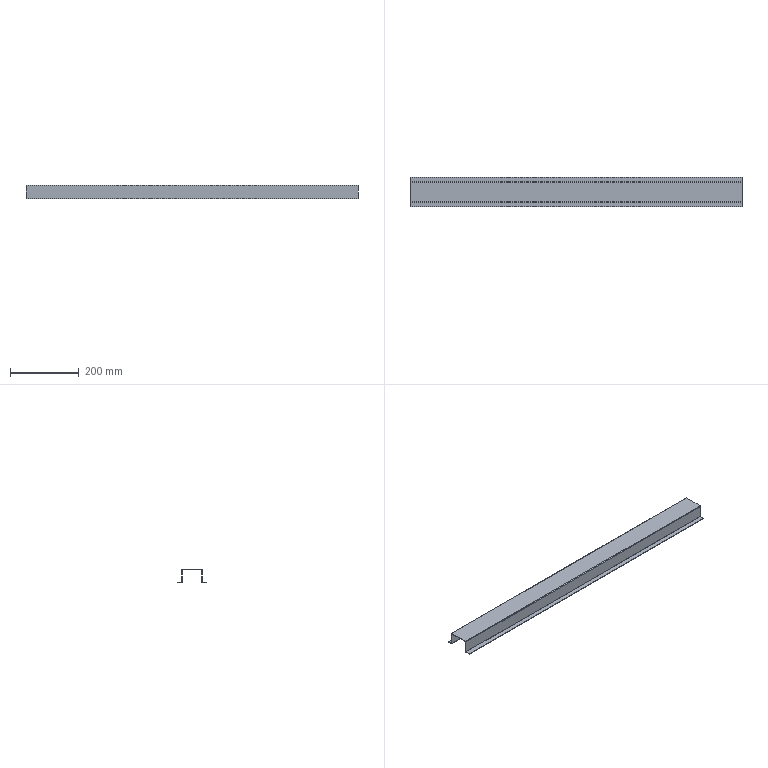Part | STEP file | FHD-021-001-S rack welded part S | 1 solid | 22 faces | box 969 x 87 x 38.5 mm | volume 231643 mm3 | plane 14 | cylinder 8 | commonest cylinder face diameters 0.4 x4 3.4 x4